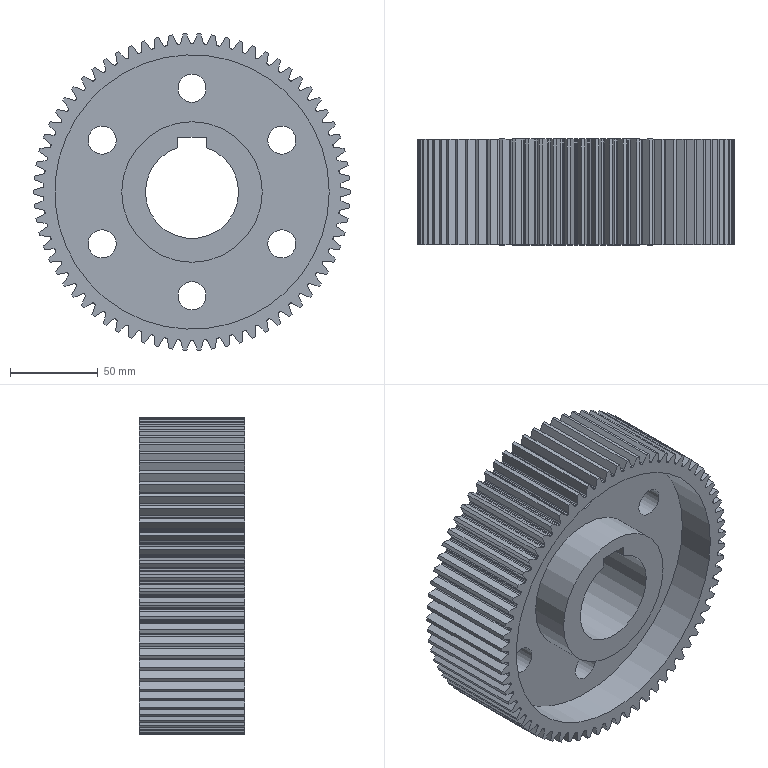Part | NX | features BREP 70, META 70, EXTRACT_DATUM_AXIS 14, DATUM_CSYS 10, EXTRUDE 9, SKETCH 9, EXTRACT_DATUM_PLANE 8, EXTRACT_STRING 8, Instance Feature 6, CYLINDER 1, FSET 1, Mirror Feature 1, Pattern Feature 1 | 1 solid | 440 faces | box 180 x 60 x 179.897 mm | volume 648529 mm3 | spline 350 | cylinder 81 | plane 9 | commonest cylinder face diameters 168.75 x70 16 x6 80 x2 156 x2 53 x1